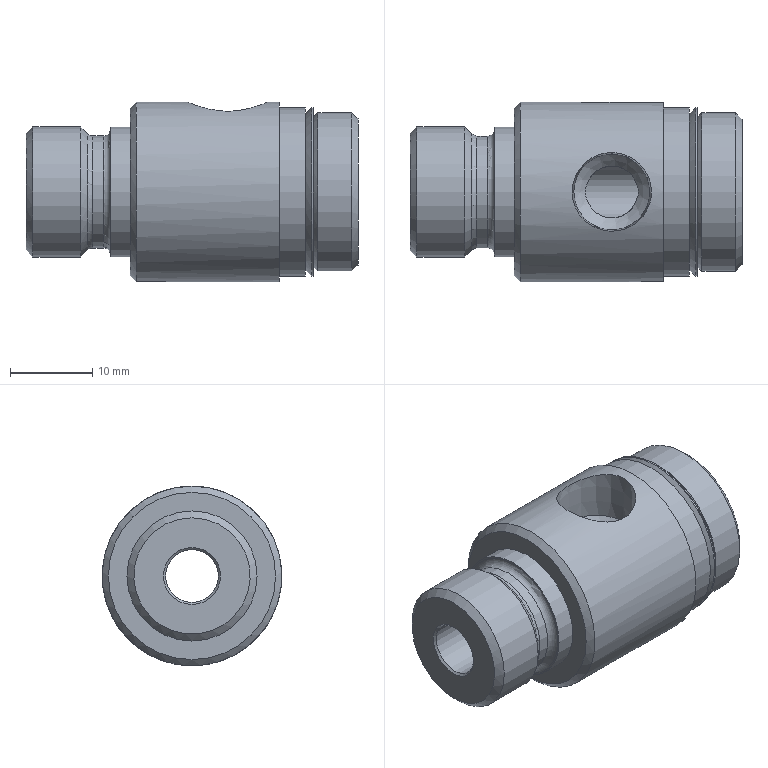Part | NX | features solid 2 | 1 solid | 32 faces | box 40.488 x 21.908 x 21.908 mm | volume 10238 mm3 | cylinder 11 | cone 11 | plane 7 | torus 3 | commonest cylinder face diameters 6.35 x2 20.511 x2 6.439 x1 13.678 x1 15.812 x1 15.875 x1
STEP:
#1=CARTESIAN_POINT('',(34.074,0.,10.255));
#2=VERTEX_POINT('',#1);
#3=CARTESIAN_POINT('',(34.074,0.,0.));
#4=DIRECTION('',(-1.,0.,0.));
#5=DIRECTION('',(0.,0.,1.));
#6=AXIS2_PLACEMENT_3D('',#3,#4,#5);
#7=CIRCLE('',#6,10.255);
#8=EDGE_CURVE('',#2,#2,#7,.T.);
#9=ORIENTED_EDGE('',*,*,#8,.F.);
#10=EDGE_LOOP('',(#9));
#11=FACE_BOUND('',#10,.T.);
#12=CARTESIAN_POINT('',(34.074,0.,9.512));
#13=VERTEX_POINT('',#12);
#14=CARTESIAN_POINT('',(34.074,0.,0.));
#15=DIRECTION('',(-1.,0.,0.));
#16=DIRECTION('',(0.,0.,1.));
#17=AXIS2_PLACEMENT_3D('',#14,#15,#16);
#18=CIRCLE('',#17,9.512);
#19=EDGE_CURVE('',#13,#13,#18,.T.);
#20=ORIENTED_EDGE('',*,*,#19,.T.);
#21=EDGE_LOOP('',(#20));
#22=FACE_BOUND('',#21,.T.);
#23=CARTESIAN_POINT('',(34.074,10.954,0.));
#24=DIRECTION('',(1.,0.,0.));
#25=DIRECTION('',(0.,0.,-1.));
#26=AXIS2_PLACEMENT_3D('',#23,#24,#25);
#27=PLANE('',#26);
#28=ADVANCED_FACE('',(#11,#22),#27,.T.);
#29=CARTESIAN_POINT('',(34.836,0.,8.909));
#30=VERTEX_POINT('',#29);
#31=CARTESIAN_POINT('',(34.836,0.,0.));
#32=DIRECTION('',(-1.,0.,0.));
#33=DIRECTION('',(0.,0.,1.));
#34=AXIS2_PLACEMENT_3D('',#31,#32,#33);
#35=CIRCLE('',#34,8.909);
#36=EDGE_CURVE('',#30,#30,#35,.T.);
#37=ORIENTED_EDGE('',*,*,#36,.T.);
#38=EDGE_LOOP('',(#37));
#39=FACE_BOUND('',#38,.T.);
#40=CARTESIAN_POINT('',(34.455,0.,8.909));
#41=VERTEX_POINT('',#40);
#42=CARTESIAN_POINT('',(34.455,0.,0.));
#43=DIRECTION('',(-1.,0.,0.));
#44=DIRECTION('',(0.,0.,1.));
#45=AXIS2_PLACEMENT_3D('',#42,#43,#44);
#46=CIRCLE('',#45,8.909);
#47=EDGE_CURVE('',#41,#41,#46,.T.);
#48=ORIENTED_EDGE('',*,*,#47,.F.);
#49=EDGE_LOOP('',(#48));
#50=FACE_BOUND('',#49,.T.);
#51=CARTESIAN_POINT('',(40.488,0.,0.));
#52=DIRECTION('',(-1.,0.,0.));
#53=DIRECTION('',(0.,0.,1.));
#54=AXIS2_PLACEMENT_3D('',#51,#52,#53);
#55=CYLINDRICAL_SURFACE('',#54,8.909);
#56=ADVANCED_FACE('',(#39,#50),#55,.T.);
#57=CARTESIAN_POINT('',(21.396,-3.591,10.349));
#58=VERTEX_POINT('',#57);
#59=CARTESIAN_POINT('',(19.251,-0.2976,11.215));
#60=CARTESIAN_POINT('',(21.051,-3.985,10.329));
#61=CARTESIAN_POINT('',(24.92,-5.307,9.56));
#62=CARTESIAN_POINT('',(28.595,-3.568,10.515));
#63=CARTESIAN_POINT('',(29.973,0.3053,11.214));
#64=CARTESIAN_POINT('',(28.18,3.975,10.332));
#65=CARTESIAN_POINT('',(24.314,5.311,9.559));
#66=CARTESIAN_POINT('',(20.63,3.567,10.514));
#67=CARTESIAN_POINT('',(19.251,-0.2976,11.215));
#68=CARTESIAN_POINT('',(21.051,-3.985,10.329));
#69=CARTESIAN_POINT('',(24.92,-5.307,9.56));
#70=B_SPLINE_CURVE_WITH_KNOTS('',3,(#59,#60,#61,#62,#63,#64,#65,#66,#67,#68,#69),.UNSPECIFIED.,.T.,.F.,(1,1,1,1,1,1,1,1,1,1,1,1,1,1,1),(-0.01145,-0.007634,-0.003817,0.,0.003817,0.007634,0.01145,0.01527,0.01909,0.0229,0.02672,0.03054,0.03436,0.03817,0.04199),.UNSPECIFIED.);
#71=EDGE_CURVE('',#58,#58,#70,.T.);
#72=ORIENTED_EDGE('',*,*,#71,.F.);
#73=EDGE_LOOP('',(#72));
#74=FACE_BOUND('',#73,.T.);
#75=CARTESIAN_POINT('',(13.462,0.,10.954));
#76=VERTEX_POINT('',#75);
#77=CARTESIAN_POINT('',(13.462,0.,0.));
#78=DIRECTION('',(-1.,0.,0.));
#79=DIRECTION('',(0.,0.,1.));
#80=AXIS2_PLACEMENT_3D('',#77,#78,#79);
#81=CIRCLE('',#80,10.954);
#82=EDGE_CURVE('',#76,#76,#81,.T.);
#83=ORIENTED_EDGE('',*,*,#82,.F.);
#84=EDGE_LOOP('',(#83));
#85=FACE_BOUND('',#84,.T.);
#86=CARTESIAN_POINT('',(30.899,0.,-10.954));
#87=VERTEX_POINT('',#86);
#88=CARTESIAN_POINT('',(30.899,0.,0.));
#89=DIRECTION('',(1.,0.,0.));
#90=DIRECTION('',(0.,0.,-1.));
#91=AXIS2_PLACEMENT_3D('',#88,#89,#90);
#92=CIRCLE('',#91,10.954);
#93=EDGE_CURVE('',#87,#87,#92,.F.);
#94=ORIENTED_EDGE('',*,*,#93,.T.);
#95=EDGE_LOOP('',(#94));
#96=FACE_BOUND('',#95,.T.);
#97=CARTESIAN_POINT('',(40.488,0.,0.));
#98=DIRECTION('',(-1.,0.,0.));
#99=DIRECTION('',(0.,0.,1.));
#100=AXIS2_PLACEMENT_3D('',#97,#98,#99);
#101=CYLINDRICAL_SURFACE('',#100,10.954);
#102=ADVANCED_FACE('',(#74,#85,#96),#101,.T.);
#103=CARTESIAN_POINT('',(7.52,0.,7.097));
#104=VERTEX_POINT('',#103);
#105=CARTESIAN_POINT('',(7.52,0.,0.));
#106=DIRECTION('',(-1.,0.,0.));
#107=DIRECTION('',(0.,0.,1.));
#108=AXIS2_PLACEMENT_3D('',#105,#106,#107);
#109=CIRCLE('',#108,7.097);
#110=EDGE_CURVE('',#104,#104,#109,.T.);
#111=ORIENTED_EDGE('',*,*,#110,.T.);
#112=EDGE_LOOP('',(#111));
#113=FACE_BOUND('',#112,.T.);
#114=CARTESIAN_POINT('',(6.682,0.,7.938));
#115=VERTEX_POINT('',#114);
#116=CARTESIAN_POINT('',(6.682,0.,0.));
#117=DIRECTION('',(-1.,0.,0.));
#118=DIRECTION('',(0.,0.,1.));
#119=AXIS2_PLACEMENT_3D('',#116,#117,#118);
#120=CIRCLE('',#119,7.938);
#121=EDGE_CURVE('',#115,#115,#120,.T.);
#122=ORIENTED_EDGE('',*,*,#121,.F.);
#123=EDGE_LOOP('',(#122));
#124=FACE_BOUND('',#123,.T.);
#125=CARTESIAN_POINT('',(6.682,0.,0.));
#126=DIRECTION('',(-1.,0.,0.));
#127=DIRECTION('',(0.,0.,1.));
#128=AXIS2_PLACEMENT_3D('',#125,#126,#127);
#129=CONICAL_SURFACE('',#128,7.938,0.7868);
#130=ADVANCED_FACE('',(#113,#124),#129,.T.);
#131=ORIENTED_EDGE('',*,*,#110,.F.);
#132=EDGE_LOOP('',(#131));
#133=FACE_BOUND('',#132,.T.);
#134=CARTESIAN_POINT('',(8.141,0.,6.839));
#135=VERTEX_POINT('',#134);
#136=CARTESIAN_POINT('',(8.141,0.,0.));
#137=DIRECTION('',(-1.,0.,0.));
#138=DIRECTION('',(0.,0.,1.));
#139=AXIS2_PLACEMENT_3D('',#136,#137,#138);
#140=CIRCLE('',#139,6.839);
#141=EDGE_CURVE('',#135,#135,#140,.T.);
#142=ORIENTED_EDGE('',*,*,#141,.T.);
#143=EDGE_LOOP('',(#142));
#144=FACE_BOUND('',#143,.T.);
#145=CARTESIAN_POINT('',(8.141,0.,0.));
#146=DIRECTION('',(-1.,0.,0.));
#147=DIRECTION('',(0.,0.,1.));
#148=AXIS2_PLACEMENT_3D('',#145,#146,#147);
#149=TOROIDAL_SURFACE('',#148,7.715,0.8763);
#150=ADVANCED_FACE('',(#133,#144),#149,.F.);
#151=CARTESIAN_POINT('',(9.436,0.,6.839));
#152=VERTEX_POINT('',#151);
#153=CARTESIAN_POINT('',(9.436,0.,0.));
#154=DIRECTION('',(-1.,0.,0.));
#155=DIRECTION('',(0.,0.,1.));
#156=AXIS2_PLACEMENT_3D('',#153,#154,#155);
#157=CIRCLE('',#156,6.839);
#158=EDGE_CURVE('',#152,#152,#157,.T.);
#159=ORIENTED_EDGE('',*,*,#158,.T.);
#160=EDGE_LOOP('',(#159));
#161=FACE_BOUND('',#160,.T.);
#162=ORIENTED_EDGE('',*,*,#141,.F.);
#163=EDGE_LOOP('',(#162));
#164=FACE_BOUND('',#163,.T.);
#165=CARTESIAN_POINT('',(12.7,0.,0.));
#166=DIRECTION('',(-1.,0.,0.));
#167=DIRECTION('',(0.,0.,1.));
#168=AXIS2_PLACEMENT_3D('',#165,#166,#167);
#169=CYLINDRICAL_SURFACE('',#168,6.839);
#170=ADVANCED_FACE('',(#161,#164),#169,.T.);
#171=ORIENTED_EDGE('',*,*,#158,.F.);
#172=EDGE_LOOP('',(#171));
#173=FACE_BOUND('',#172,.T.);
#174=CARTESIAN_POINT('',(10.312,0.,7.715));
#175=VERTEX_POINT('',#174);
#176=CARTESIAN_POINT('',(10.312,0.,0.));
#177=DIRECTION('',(-1.,0.,0.));
#178=DIRECTION('',(0.,0.,1.));
#179=AXIS2_PLACEMENT_3D('',#176,#177,#178);
#180=CIRCLE('',#179,7.715);
#181=EDGE_CURVE('',#175,#175,#180,.T.);
#182=ORIENTED_EDGE('',*,*,#181,.T.);
#183=EDGE_LOOP('',(#182));
#184=FACE_BOUND('',#183,.T.);
#185=CARTESIAN_POINT('',(9.436,0.,0.));
#186=DIRECTION('',(-1.,0.,0.));
#187=DIRECTION('',(0.,0.,1.));
#188=AXIS2_PLACEMENT_3D('',#185,#186,#187);
#189=TOROIDAL_SURFACE('',#188,7.715,0.8763);
#190=ADVANCED_FACE('',(#173,#184),#189,.F.);
#191=CARTESIAN_POINT('',(10.312,0.,7.906));
#192=VERTEX_POINT('',#191);
#193=CARTESIAN_POINT('',(10.312,0.,0.));
#194=DIRECTION('',(-1.,0.,0.));
#195=DIRECTION('',(0.,0.,1.));
#196=AXIS2_PLACEMENT_3D('',#193,#194,#195);
#197=CIRCLE('',#196,7.906);
#198=EDGE_CURVE('',#192,#192,#197,.T.);
#199=ORIENTED_EDGE('',*,*,#198,.T.);
#200=EDGE_LOOP('',(#199));
#201=FACE_BOUND('',#200,.T.);
#202=ORIENTED_EDGE('',*,*,#181,.F.);
#203=EDGE_LOOP('',(#202));
#204=FACE_BOUND('',#203,.T.);
#205=CARTESIAN_POINT('',(10.312,7.715,0.));
#206=DIRECTION('',(-1.,0.,0.));
#207=DIRECTION('',(0.,0.,1.));
#208=AXIS2_PLACEMENT_3D('',#205,#206,#207);
#209=PLANE('',#208);
#210=ADVANCED_FACE('',(#201,#204),#209,.T.);
#211=CARTESIAN_POINT('',(12.7,0.,7.906));
#212=VERTEX_POINT('',#211);
#213=CARTESIAN_POINT('',(12.7,0.,0.));
#214=DIRECTION('',(-1.,0.,0.));
#215=DIRECTION('',(0.,0.,1.));
#216=AXIS2_PLACEMENT_3D('',#213,#214,#215);
#217=CIRCLE('',#216,7.906);
#218=EDGE_CURVE('',#212,#212,#217,.F.);
#219=ORIENTED_EDGE('',*,*,#218,.F.);
#220=EDGE_LOOP('',(#219));
#221=FACE_BOUND('',#220,.T.);
#222=ORIENTED_EDGE('',*,*,#198,.F.);
#223=EDGE_LOOP('',(#222));
#224=FACE_BOUND('',#223,.T.);
#225=CARTESIAN_POINT('',(12.7,0.,0.));
#226=DIRECTION('',(-1.,0.,0.));
#227=DIRECTION('',(0.,0.,1.));
#228=AXIS2_PLACEMENT_3D('',#225,#226,#227);
#229=CYLINDRICAL_SURFACE('',#228,7.906);
#230=ADVANCED_FACE('',(#221,#224),#229,.T.);
#231=CARTESIAN_POINT('',(0.,0.,-3.473));
#232=VERTEX_POINT('',#231);
#233=CARTESIAN_POINT('',(0.,0.,0.));
#234=DIRECTION('',(1.,0.,0.));
#235=DIRECTION('',(0.,0.,-1.));
#236=AXIS2_PLACEMENT_3D('',#233,#234,#235);
#237=CIRCLE('',#236,3.473);
#238=EDGE_CURVE('',#232,#232,#237,.T.);
#239=ORIENTED_EDGE('',*,*,#238,.T.);
#240=EDGE_LOOP('',(#239));
#241=FACE_BOUND('',#240,.T.);
#242=CARTESIAN_POINT('',(0.,0.,7.098));
#243=VERTEX_POINT('',#242);
#244=CARTESIAN_POINT('',(0.,0.,0.));
#245=DIRECTION('',(-1.,0.,0.));
#246=DIRECTION('',(0.,0.,1.));
#247=AXIS2_PLACEMENT_3D('',#244,#245,#246);
#248=CIRCLE('',#247,7.098);
#249=EDGE_CURVE('',#243,#243,#248,.T.);
#250=ORIENTED_EDGE('',*,*,#249,.T.);
#251=EDGE_LOOP('',(#250));
#252=FACE_BOUND('',#251,.T.);
#253=CARTESIAN_POINT('',(0.,0.,0.));
#254=DIRECTION('',(-1.,0.,0.));
#255=DIRECTION('',(0.,0.,1.));
#256=AXIS2_PLACEMENT_3D('',#253,#254,#255);
#257=PLANE('',#256);
#258=ADVANCED_FACE('',(#241,#252),#257,.T.);
#259=CARTESIAN_POINT('',(0.8395,0.,7.938));
#260=VERTEX_POINT('',#259);
#261=CARTESIAN_POINT('',(0.8395,0.,0.));
#262=DIRECTION('',(-1.,0.,0.));
#263=DIRECTION('',(0.,0.,1.));
#264=AXIS2_PLACEMENT_3D('',#261,#262,#263);
#265=CIRCLE('',#264,7.938);
#266=EDGE_CURVE('',#260,#260,#265,.T.);
#267=ORIENTED_EDGE('',*,*,#266,.T.);
#268=EDGE_LOOP('',(#267));
#269=FACE_BOUND('',#268,.T.);
#270=ORIENTED_EDGE('',*,*,#249,.F.);
#271=EDGE_LOOP('',(#270));
#272=FACE_BOUND('',#271,.T.);
#273=CARTESIAN_POINT('',(0.,0.,0.));
#274=DIRECTION('',(1.,0.,0.));
#275=DIRECTION('',(0.,0.,-1.));
#276=AXIS2_PLACEMENT_3D('',#273,#274,#275);
#277=CONICAL_SURFACE('',#276,7.098,0.7854);
#278=ADVANCED_FACE('',(#269,#272),#277,.T.);
#279=ORIENTED_EDGE('',*,*,#121,.T.);
#280=EDGE_LOOP('',(#279));
#281=FACE_BOUND('',#280,.T.);
#282=ORIENTED_EDGE('',*,*,#266,.F.);
#283=EDGE_LOOP('',(#282));
#284=FACE_BOUND('',#283,.T.);
#285=CARTESIAN_POINT('',(12.7,0.,0.));
#286=DIRECTION('',(-1.,0.,0.));
#287=DIRECTION('',(0.,0.,1.));
#288=AXIS2_PLACEMENT_3D('',#285,#286,#287);
#289=CYLINDRICAL_SURFACE('',#288,7.938);
#290=ADVANCED_FACE('',(#281,#284),#289,.T.);
#291=CARTESIAN_POINT('',(40.488,0.,-3.219));
#292=VERTEX_POINT('',#291);
#293=CARTESIAN_POINT('',(40.488,0.,0.));
#294=DIRECTION('',(1.,0.,0.));
#295=DIRECTION('',(0.,0.,-1.));
#296=AXIS2_PLACEMENT_3D('',#293,#294,#295);
#297=CIRCLE('',#296,3.219);
#298=EDGE_CURVE('',#292,#292,#297,.T.);
#299=ORIENTED_EDGE('',*,*,#298,.F.);
#300=EDGE_LOOP('',(#299));
#301=FACE_BOUND('',#300,.T.);
#302=CARTESIAN_POINT('',(40.488,0.,8.909));
#303=VERTEX_POINT('',#302);
#304=CARTESIAN_POINT('',(40.488,0.,0.));
#305=DIRECTION('',(-1.,0.,0.));
#306=DIRECTION('',(0.,0.,1.));
#307=AXIS2_PLACEMENT_3D('',#304,#305,#306);
#308=CIRCLE('',#307,8.909);
#309=EDGE_CURVE('',#303,#303,#308,.T.);
#310=ORIENTED_EDGE('',*,*,#309,.F.);
#311=EDGE_LOOP('',(#310));
#312=FACE_BOUND('',#311,.T.);
#313=CARTESIAN_POINT('',(40.488,8.909,0.));
#314=DIRECTION('',(1.,0.,0.));
#315=DIRECTION('',(0.,0.,-1.));
#316=AXIS2_PLACEMENT_3D('',#313,#314,#315);
#317=PLANE('',#316);
#318=ADVANCED_FACE('',(#301,#312),#317,.T.);
#319=ORIENTED_EDGE('',*,*,#218,.T.);
#320=EDGE_LOOP('',(#319));
#321=FACE_BOUND('',#320,.T.);
#322=CARTESIAN_POINT('',(12.7,0.,10.192));
#323=VERTEX_POINT('',#322);
#324=CARTESIAN_POINT('',(12.7,0.,0.));
#325=DIRECTION('',(-1.,0.,0.));
#326=DIRECTION('',(0.,0.,1.));
#327=AXIS2_PLACEMENT_3D('',#324,#325,#326);
#328=CIRCLE('',#327,10.192);
#329=EDGE_CURVE('',#323,#323,#328,.T.);
#330=ORIENTED_EDGE('',*,*,#329,.T.);
#331=EDGE_LOOP('',(#330));
#332=FACE_BOUND('',#331,.T.);
#333=CARTESIAN_POINT('',(12.7,0.,0.));
#334=DIRECTION('',(-1.,0.,0.));
#335=DIRECTION('',(0.,0.,1.));
#336=AXIS2_PLACEMENT_3D('',#333,#334,#335);
#337=PLANE('',#336);
#338=ADVANCED_FACE('',(#321,#332),#337,.T.);
#339=ORIENTED_EDGE('',*,*,#82,.T.);
#340=EDGE_LOOP('',(#339));
#341=FACE_BOUND('',#340,.T.);
#342=ORIENTED_EDGE('',*,*,#329,.F.);
#343=EDGE_LOOP('',(#342));
#344=FACE_BOUND('',#343,.T.);
#345=CARTESIAN_POINT('',(12.7,0.,0.));
#346=DIRECTION('',(1.,0.,0.));
#347=DIRECTION('',(0.,0.,-1.));
#348=AXIS2_PLACEMENT_3D('',#345,#346,#347);
#349=CONICAL_SURFACE('',#348,10.192,0.7854);
#350=ADVANCED_FACE('',(#341,#344),#349,.T.);
#351=CARTESIAN_POINT('',(35.598,0.,9.671));
#352=VERTEX_POINT('',#351);
#353=CARTESIAN_POINT('',(35.598,0.,0.));
#354=DIRECTION('',(-1.,0.,0.));
#355=DIRECTION('',(0.,0.,1.));
#356=AXIS2_PLACEMENT_3D('',#353,#354,#355);
#357=CIRCLE('',#356,9.671);
#358=EDGE_CURVE('',#352,#352,#357,.T.);
#359=ORIENTED_EDGE('',*,*,#358,.T.);
#360=EDGE_LOOP('',(#359));
#361=FACE_BOUND('',#360,.T.);
#362=ORIENTED_EDGE('',*,*,#36,.F.);
#363=EDGE_LOOP('',(#362));
#364=FACE_BOUND('',#363,.T.);
#365=CARTESIAN_POINT('',(34.836,0.,0.));
#366=DIRECTION('',(1.,0.,0.));
#367=DIRECTION('',(0.,0.,-1.));
#368=AXIS2_PLACEMENT_3D('',#365,#366,#367);
#369=CONICAL_SURFACE('',#368,8.909,0.7854);
#370=ADVANCED_FACE('',(#361,#364),#369,.T.);
#371=CARTESIAN_POINT('',(39.726,0.,9.671));
#372=VERTEX_POINT('',#371);
#373=CARTESIAN_POINT('',(39.726,0.,0.));
#374=DIRECTION('',(-1.,0.,0.));
#375=DIRECTION('',(0.,0.,1.));
#376=AXIS2_PLACEMENT_3D('',#373,#374,#375);
#377=CIRCLE('',#376,9.671);
#378=EDGE_CURVE('',#372,#372,#377,.T.);
#379=ORIENTED_EDGE('',*,*,#378,.T.);
#380=EDGE_LOOP('',(#379));
#381=FACE_BOUND('',#380,.T.);
#382=ORIENTED_EDGE('',*,*,#358,.F.);
#383=EDGE_LOOP('',(#382));
#384=FACE_BOUND('',#383,.T.);
#385=CARTESIAN_POINT('',(40.488,0.,0.));
#386=DIRECTION('',(-1.,0.,0.));
#387=DIRECTION('',(0.,0.,1.));
#388=AXIS2_PLACEMENT_3D('',#385,#386,#387);
#389=CYLINDRICAL_SURFACE('',#388,9.671);
#390=ADVANCED_FACE('',(#381,#384),#389,.T.);
#391=ORIENTED_EDGE('',*,*,#309,.T.);
#392=EDGE_LOOP('',(#391));
#393=FACE_BOUND('',#392,.T.);
#394=ORIENTED_EDGE('',*,*,#378,.F.);
#395=EDGE_LOOP('',(#394));
#396=FACE_BOUND('',#395,.T.);
#397=CARTESIAN_POINT('',(39.726,0.,0.));
#398=DIRECTION('',(-1.,0.,0.));
#399=DIRECTION('',(0.,0.,1.));
#400=AXIS2_PLACEMENT_3D('',#397,#398,#399);
#401=CONICAL_SURFACE('',#400,9.671,0.7854);
#402=ADVANCED_FACE('',(#393,#396),#401,.T.);
#403=CARTESIAN_POINT('',(21.521,-0.7217,3.138));
#404=VERTEX_POINT('',#403);
#405=CARTESIAN_POINT('',(27.704,-0.7217,3.138));
#406=VERTEX_POINT('',#405);
#407=CARTESIAN_POINT('',(21.521,-0.7217,3.138));
#408=CARTESIAN_POINT('',(21.615,-1.128,3.044));
#409=CARTESIAN_POINT('',(21.951,-1.845,2.714));
#410=CARTESIAN_POINT('',(22.694,-2.595,1.987));
#411=CARTESIAN_POINT('',(23.412,-2.967,1.306));
#412=CARTESIAN_POINT('',(24.026,-3.136,0.7681));
#413=CARTESIAN_POINT('',(24.623,-3.195,0.4125));
#414=CARTESIAN_POINT('',(25.213,-3.133,0.7813));
#415=CARTESIAN_POINT('',(25.818,-2.965,1.309));
#416=CARTESIAN_POINT('',(26.538,-2.59,1.995));
#417=CARTESIAN_POINT('',(27.274,-1.845,2.713));
#418=CARTESIAN_POINT('',(27.61,-1.125,3.045));
#419=CARTESIAN_POINT('',(27.704,-0.7217,3.138));
#420=B_SPLINE_CURVE_WITH_KNOTS('',3,(#407,#408,#409,#410,#411,#412,#413,#414,#415,#416,#417,#418,#419),.UNSPECIFIED.,.F.,.F.,(4,1,1,1,1,1,1,1,1,1,4),(0.,0.001258,0.002517,0.003775,0.004405,0.005034,0.005663,0.006292,0.007551,0.008809,0.01007),.UNSPECIFIED.);
#421=EDGE_CURVE('',#404,#406,#420,.T.);
#422=ORIENTED_EDGE('',*,*,#421,.T.);
#423=CARTESIAN_POINT('',(27.704,0.7217,3.138));
#424=VERTEX_POINT('',#423);
#425=CARTESIAN_POINT('',(27.704,-0.7217,3.138));
#426=CARTESIAN_POINT('',(27.914,-0.2749,3.24));
#427=CARTESIAN_POINT('',(27.914,0.275,3.24));
#428=CARTESIAN_POINT('',(27.704,0.7217,3.138));
#429=B_SPLINE_CURVE_WITH_KNOTS('',3,(#425,#426,#427,#428),.UNSPECIFIED.,.F.,.F.,(4,4),(0.00003996,0.001539),.UNSPECIFIED.);
#430=EDGE_CURVE('',#406,#424,#429,.T.);
#431=ORIENTED_EDGE('',*,*,#430,.T.);
#432=CARTESIAN_POINT('',(21.521,0.7217,3.138));
#433=VERTEX_POINT('',#432);
#434=CARTESIAN_POINT('',(27.704,0.7217,3.138));
#435=CARTESIAN_POINT('',(27.61,1.128,3.044));
#436=CARTESIAN_POINT('',(27.274,1.845,2.714));
#437=CARTESIAN_POINT('',(26.531,2.595,1.987));
#438=CARTESIAN_POINT('',(25.813,2.967,1.306));
#439=CARTESIAN_POINT('',(25.199,3.136,0.7681));
#440=CARTESIAN_POINT('',(24.603,3.195,0.4125));
#441=CARTESIAN_POINT('',(24.013,3.133,0.7813));
#442=CARTESIAN_POINT('',(23.407,2.965,1.309));
#443=CARTESIAN_POINT('',(22.687,2.59,1.995));
#444=CARTESIAN_POINT('',(21.951,1.845,2.713));
#445=CARTESIAN_POINT('',(21.615,1.125,3.045));
#446=CARTESIAN_POINT('',(21.521,0.7217,3.138));
#447=B_SPLINE_CURVE_WITH_KNOTS('',3,(#434,#435,#436,#437,#438,#439,#440,#441,#442,#443,#444,#445,#446),.UNSPECIFIED.,.F.,.F.,(4,1,1,1,1,1,1,1,1,1,4),(0.,0.001258,0.002517,0.003775,0.004405,0.005034,0.005663,0.006292,0.007551,0.008809,0.01007),.UNSPECIFIED.);
#448=EDGE_CURVE('',#424,#433,#447,.T.);
#449=ORIENTED_EDGE('',*,*,#448,.T.);
#450=CARTESIAN_POINT('',(21.521,0.7217,3.138));
#451=CARTESIAN_POINT('',(21.311,0.2749,3.24));
#452=CARTESIAN_POINT('',(21.311,-0.275,3.24));
#453=CARTESIAN_POINT('',(21.521,-0.7217,3.138));
#454=B_SPLINE_CURVE_WITH_KNOTS('',3,(#450,#451,#452,#453),.UNSPECIFIED.,.F.,.F.,(4,4),(0.00003996,0.001539),.UNSPECIFIED.);
#455=EDGE_CURVE('',#433,#404,#454,.T.);
#456=ORIENTED_EDGE('',*,*,#455,.T.);
#457=EDGE_LOOP('',(#422,#431,#449,#456));
#458=FACE_BOUND('',#457,.T.);
#459=ORIENTED_EDGE('',*,*,#298,.T.);
#460=EDGE_LOOP('',(#459));
#461=FACE_BOUND('',#460,.T.);
#462=CARTESIAN_POINT('',(0.254,0.,-3.219));
#463=VERTEX_POINT('',#462);
#464=CARTESIAN_POINT('',(0.254,0.,0.));
#465=DIRECTION('',(1.,0.,0.));
#466=DIRECTION('',(0.,0.,-1.));
#467=AXIS2_PLACEMENT_3D('',#464,#465,#466);
#468=CIRCLE('',#467,3.219);
#469=EDGE_CURVE('',#463,#463,#468,.T.);
#470=ORIENTED_EDGE('',*,*,#469,.F.);
#471=EDGE_LOOP('',(#470));
#472=FACE_BOUND('',#471,.T.);
#473=CARTESIAN_POINT('',(40.488,0.,0.));
#474=DIRECTION('',(1.,0.,0.));
#475=DIRECTION('',(0.,0.,-1.));
#476=AXIS2_PLACEMENT_3D('',#473,#474,#475);
#477=CYLINDRICAL_SURFACE('',#476,3.219);
#478=ADVANCED_FACE('',(#458,#461,#472),#477,.F.);
#479=ORIENTED_EDGE('',*,*,#469,.T.);
#480=EDGE_LOOP('',(#479));
#481=FACE_BOUND('',#480,.T.);
#482=ORIENTED_EDGE('',*,*,#238,.F.);
#483=EDGE_LOOP('',(#482));
#484=FACE_BOUND('',#483,.T.);
#485=CARTESIAN_POINT('',(0.,0.,0.));
#486=DIRECTION('',(-1.,0.,0.));
#487=DIRECTION('',(0.,0.,1.));
#488=AXIS2_PLACEMENT_3D('',#485,#486,#487);
#489=CONICAL_SURFACE('',#488,3.473,0.7854);
#490=ADVANCED_FACE('',(#481,#484),#489,.F.);
#491=ORIENTED_EDGE('',*,*,#93,.F.);
#492=EDGE_LOOP('',(#491));
#493=FACE_BOUND('',#492,.T.);
#494=CARTESIAN_POINT('',(30.899,0.,10.255));
#495=VERTEX_POINT('',#494);
#496=CARTESIAN_POINT('',(30.899,0.,0.));
#497=DIRECTION('',(-1.,0.,0.));
#498=DIRECTION('',(0.,0.,1.));
#499=AXIS2_PLACEMENT_3D('',#496,#497,#498);
#500=CIRCLE('',#499,10.255);
#501=EDGE_CURVE('',#495,#495,#500,.T.);
#502=ORIENTED_EDGE('',*,*,#501,.T.);
#503=EDGE_LOOP('',(#502));
#504=FACE_BOUND('',#503,.T.);
#505=CARTESIAN_POINT('',(30.899,15.335,0.));
#506=DIRECTION('',(1.,0.,0.));
#507=DIRECTION('',(0.,0.,-1.));
#508=AXIS2_PLACEMENT_3D('',#505,#506,#507);
#509=PLANE('',#508);
#510=ADVANCED_FACE('',(#493,#504),#509,.T.);
#511=ORIENTED_EDGE('',*,*,#8,.T.);
#512=EDGE_LOOP('',(#511));
#513=FACE_BOUND('',#512,.T.);
#514=ORIENTED_EDGE('',*,*,#501,.F.);
#515=EDGE_LOOP('',(#514));
#516=FACE_BOUND('',#515,.T.);
#517=CARTESIAN_POINT('',(34.074,0.,0.));
#518=DIRECTION('',(-1.,0.,0.));
#519=DIRECTION('',(0.,0.,1.));
#520=AXIS2_PLACEMENT_3D('',#517,#518,#519);
#521=CYLINDRICAL_SURFACE('',#520,10.255);
#522=ADVANCED_FACE('',(#513,#516),#521,.T.);
#523=CARTESIAN_POINT('',(24.613,0.,3.138));
#524=DIRECTION('',(0.,0.,-1.));
#525=DIRECTION('',(-1.,0.,0.));
#526=AXIS2_PLACEMENT_3D('',#523,#524,#525);
#527=CIRCLE('',#526,3.175);
#528=EDGE_CURVE('',#433,#424,#527,.T.);
#529=ORIENTED_EDGE('',*,*,#528,.F.);
#530=ORIENTED_EDGE('',*,*,#448,.F.);
#531=EDGE_LOOP('',(#529,#530));
#532=FACE_BOUND('',#531,.T.);
#533=CARTESIAN_POINT('',(24.613,0.,10.954));
#534=DIRECTION('',(0.,0.,-1.));
#535=DIRECTION('',(-1.,0.,0.));
#536=AXIS2_PLACEMENT_3D('',#533,#534,#535);
#537=CYLINDRICAL_SURFACE('',#536,3.175);
#538=ADVANCED_FACE('',(#532),#537,.F.);
#539=CARTESIAN_POINT('',(24.613,0.,3.138));
#540=DIRECTION('',(0.,0.,-1.));
#541=DIRECTION('',(-1.,0.,0.));
#542=AXIS2_PLACEMENT_3D('',#539,#540,#541);
#543=CIRCLE('',#542,3.175);
#544=EDGE_CURVE('',#406,#404,#543,.T.);
#545=ORIENTED_EDGE('',*,*,#544,.F.);
#546=ORIENTED_EDGE('',*,*,#421,.F.);
#547=EDGE_LOOP('',(#545,#546));
#548=FACE_BOUND('',#547,.T.);
#549=CARTESIAN_POINT('',(24.613,0.,10.954));
#550=DIRECTION('',(0.,0.,-1.));
#551=DIRECTION('',(-1.,0.,0.));
#552=AXIS2_PLACEMENT_3D('',#549,#550,#551);
#553=CYLINDRICAL_SURFACE('',#552,3.175);
#554=ADVANCED_FACE('',(#548),#553,.F.);
#555=CARTESIAN_POINT('',(19.971,0.,4.604));
#556=VERTEX_POINT('',#555);
#557=CARTESIAN_POINT('',(24.613,0.,4.604));
#558=DIRECTION('',(0.,0.,-1.));
#559=DIRECTION('',(-1.,0.,0.));
#560=AXIS2_PLACEMENT_3D('',#557,#558,#559);
#561=CIRCLE('',#560,4.641);
#562=EDGE_CURVE('',#556,#556,#561,.T.);
#563=ORIENTED_EDGE('',*,*,#562,.F.);
#564=EDGE_LOOP('',(#563));
#565=FACE_BOUND('',#564,.T.);
#566=ORIENTED_EDGE('',*,*,#544,.T.);
#567=ORIENTED_EDGE('',*,*,#455,.F.);
#568=ORIENTED_EDGE('',*,*,#528,.T.);
#569=ORIENTED_EDGE('',*,*,#430,.F.);
#570=EDGE_LOOP('',(#566,#567,#568,#569));
#571=FACE_BOUND('',#570,.T.);
#572=CARTESIAN_POINT('',(24.613,0.,3.138));
#573=DIRECTION('',(0.,0.,1.));
#574=DIRECTION('',(1.,0.,0.));
#575=AXIS2_PLACEMENT_3D('',#572,#573,#574);
#576=CONICAL_SURFACE('',#575,3.175,0.7854);
#577=ADVANCED_FACE('',(#565,#571),#576,.F.);
#578=ORIENTED_EDGE('',*,*,#71,.T.);
#579=EDGE_LOOP('',(#578));
#580=FACE_BOUND('',#579,.T.);
#581=ORIENTED_EDGE('',*,*,#562,.T.);
#582=EDGE_LOOP('',(#581));
#583=FACE_BOUND('',#582,.T.);
#584=CARTESIAN_POINT('',(24.613,0.,4.604));
#585=DIRECTION('',(0.,0.,1.));
#586=DIRECTION('',(1.,0.,0.));
#587=AXIS2_PLACEMENT_3D('',#584,#585,#586);
#588=CONICAL_SURFACE('',#587,4.641,0.03121);
#589=ADVANCED_FACE('',(#580,#583),#588,.F.);
#590=CARTESIAN_POINT('',(34.197,0.,9.168));
#591=VERTEX_POINT('',#590);
#592=CARTESIAN_POINT('',(34.197,0.,0.));
#593=DIRECTION('',(-1.,0.,0.));
#594=DIRECTION('',(0.,0.,1.));
#595=AXIS2_PLACEMENT_3D('',#592,#593,#594);
#596=CIRCLE('',#595,9.168);
#597=EDGE_CURVE('',#591,#591,#596,.T.);
#598=ORIENTED_EDGE('',*,*,#597,.F.);
#599=EDGE_LOOP('',(#598));
#600=FACE_BOUND('',#599,.T.);
#601=ORIENTED_EDGE('',*,*,#47,.T.);
#602=EDGE_LOOP('',(#601));
#603=FACE_BOUND('',#602,.T.);
#604=CARTESIAN_POINT('',(34.455,0.,0.));
#605=DIRECTION('',(-1.,0.,0.));
#606=DIRECTION('',(0.,0.,1.));
#607=AXIS2_PLACEMENT_3D('',#604,#605,#606);
#608=CONICAL_SURFACE('',#607,8.909,0.7854);
#609=ADVANCED_FACE('',(#600,#603),#608,.T.);
#610=ORIENTED_EDGE('',*,*,#597,.T.);
#611=EDGE_LOOP('',(#610));
#612=FACE_BOUND('',#611,.T.);
#613=CARTESIAN_POINT('',(34.197,0.,9.347));
#614=VERTEX_POINT('',#613);
#615=CARTESIAN_POINT('',(34.197,0.,0.));
#616=DIRECTION('',(-1.,0.,0.));
#617=DIRECTION('',(0.,0.,1.));
#618=AXIS2_PLACEMENT_3D('',#615,#616,#617);
#619=CIRCLE('',#618,9.347);
#620=EDGE_CURVE('',#614,#614,#619,.T.);
#621=ORIENTED_EDGE('',*,*,#620,.F.);
#622=EDGE_LOOP('',(#621));
#623=FACE_BOUND('',#622,.T.);
#624=CARTESIAN_POINT('',(34.286,0.,0.));
#625=DIRECTION('',(-1.,0.,0.));
#626=DIRECTION('',(0.,0.,1.));
#627=AXIS2_PLACEMENT_3D('',#624,#625,#626);
#628=TOROIDAL_SURFACE('',#627,9.257,0.127);
#629=ADVANCED_FACE('',(#612,#623),#628,.F.);
#630=CARTESIAN_POINT('',(35.021,0.,10.171));
#631=VERTEX_POINT('',#630);
#632=CARTESIAN_POINT('',(35.021,0.,0.));
#633=DIRECTION('',(-1.,0.,0.));
#634=DIRECTION('',(0.,0.,1.));
#635=AXIS2_PLACEMENT_3D('',#632,#633,#634);
#636=CIRCLE('',#635,10.171);
#637=EDGE_CURVE('',#631,#631,#636,.T.);
#638=ORIENTED_EDGE('',*,*,#637,.F.);
#639=EDGE_LOOP('',(#638));
#640=FACE_BOUND('',#639,.T.);
#641=ORIENTED_EDGE('',*,*,#620,.T.);
#642=EDGE_LOOP('',(#641));
#643=FACE_BOUND('',#642,.T.);
#644=CARTESIAN_POINT('',(34.197,0.,0.));
#645=DIRECTION('',(1.,0.,0.));
#646=DIRECTION('',(0.,0.,-1.));
#647=AXIS2_PLACEMENT_3D('',#644,#645,#646);
#648=CONICAL_SURFACE('',#647,9.347,0.7854);
#649=ADVANCED_FACE('',(#640,#643),#648,.F.);
#650=CARTESIAN_POINT('',(35.021,0.,10.255));
#651=VERTEX_POINT('',#650);
#652=CARTESIAN_POINT('',(35.021,0.,0.));
#653=DIRECTION('',(-1.,0.,0.));
#654=DIRECTION('',(0.,0.,1.));
#655=AXIS2_PLACEMENT_3D('',#652,#653,#654);
#656=CIRCLE('',#655,10.255);
#657=EDGE_CURVE('',#651,#651,#656,.T.);
#658=ORIENTED_EDGE('',*,*,#657,.F.);
#659=EDGE_LOOP('',(#658));
#660=FACE_BOUND('',#659,.T.);
#661=ORIENTED_EDGE('',*,*,#637,.T.);
#662=EDGE_LOOP('',(#661));
#663=FACE_BOUND('',#662,.T.);
#664=CARTESIAN_POINT('',(35.021,10.171,0.));
#665=DIRECTION('',(-1.,0.,0.));
#666=DIRECTION('',(0.,0.,1.));
#667=AXIS2_PLACEMENT_3D('',#664,#665,#666);
#668=PLANE('',#667);
#669=ADVANCED_FACE('',(#660,#663),#668,.F.);
#670=CARTESIAN_POINT('',(34.817,0.,10.255));
#671=VERTEX_POINT('',#670);
#672=CARTESIAN_POINT('',(34.817,0.,0.));
#673=DIRECTION('',(-1.,0.,0.));
#674=DIRECTION('',(0.,0.,1.));
#675=AXIS2_PLACEMENT_3D('',#672,#673,#674);
#676=CIRCLE('',#675,10.255);
#677=EDGE_CURVE('',#671,#671,#676,.T.);
#678=ORIENTED_EDGE('',*,*,#677,.F.);
#679=EDGE_LOOP('',(#678));
#680=FACE_BOUND('',#679,.T.);
#681=ORIENTED_EDGE('',*,*,#657,.T.);
#682=EDGE_LOOP('',(#681));
#683=FACE_BOUND('',#682,.T.);
#684=CARTESIAN_POINT('',(34.836,0.,0.));
#685=DIRECTION('',(-1.,0.,0.));
#686=DIRECTION('',(0.,0.,1.));
#687=AXIS2_PLACEMENT_3D('',#684,#685,#686);
#688=CYLINDRICAL_SURFACE('',#687,10.255);
#689=ADVANCED_FACE('',(#680,#683),#688,.T.);
#690=ORIENTED_EDGE('',*,*,#19,.F.);
#691=EDGE_LOOP('',(#690));
#692=FACE_BOUND('',#691,.T.);
#693=ORIENTED_EDGE('',*,*,#677,.T.);
#694=EDGE_LOOP('',(#693));
#695=FACE_BOUND('',#694,.T.);
#696=CARTESIAN_POINT('',(34.817,0.,0.));
#697=DIRECTION('',(1.,0.,0.));
#698=DIRECTION('',(0.,0.,-1.));
#699=AXIS2_PLACEMENT_3D('',#696,#697,#698);
#700=CONICAL_SURFACE('',#699,10.255,0.7854);
#701=ADVANCED_FACE('',(#692,#695),#700,.T.);
#702=CLOSED_SHELL('',(#28,#56,#102,#130,#150,#170,#190,#210,#230,#258,#278,#290,#318,#338,#350,#370,#390,#402,#478,#490,#510,#522,#538,#554,#577,#589,#609,#629,#649,#669,#689,#701));
#703=MANIFOLD_SOLID_BREP('',#702);
#704=(LENGTH_UNIT()NAMED_UNIT(*)SI_UNIT(.MILLI.,.METRE.));
#705=UNCERTAINTY_MEASURE_WITH_UNIT(LENGTH_MEASURE(0.0508),#704,'','');
#706=(NAMED_UNIT(*)PLANE_ANGLE_UNIT()SI_UNIT($,.RADIAN.));
#707=(NAMED_UNIT(*)SI_UNIT($,.STERADIAN.)SOLID_ANGLE_UNIT());
#708=(GEOMETRIC_REPRESENTATION_CONTEXT(3)GLOBAL_UNCERTAINTY_ASSIGNED_CONTEXT((#705))GLOBAL_UNIT_ASSIGNED_CONTEXT((#704,#706,#707))REPRESENTATION_CONTEXT('',''));
#709=ADVANCED_BREP_SHAPE_REPRESENTATION('',(#703),#708);